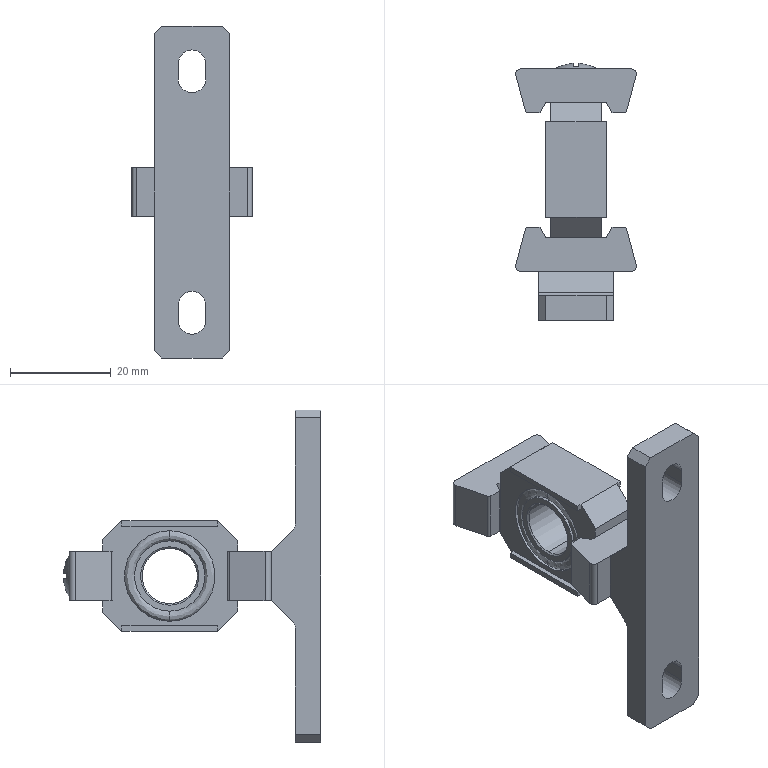Part | STEP file | 1 solid | 118 faces | box 23.994 x 51.149 x 66 mm | volume 13543 mm3 | plane 82 | cylinder 26 | spline 4 | cone 4 | other 2 | commonest cylinder face diameters 5.5 x6 1 x4 2 x4 14 x4 18 x4 4 x2